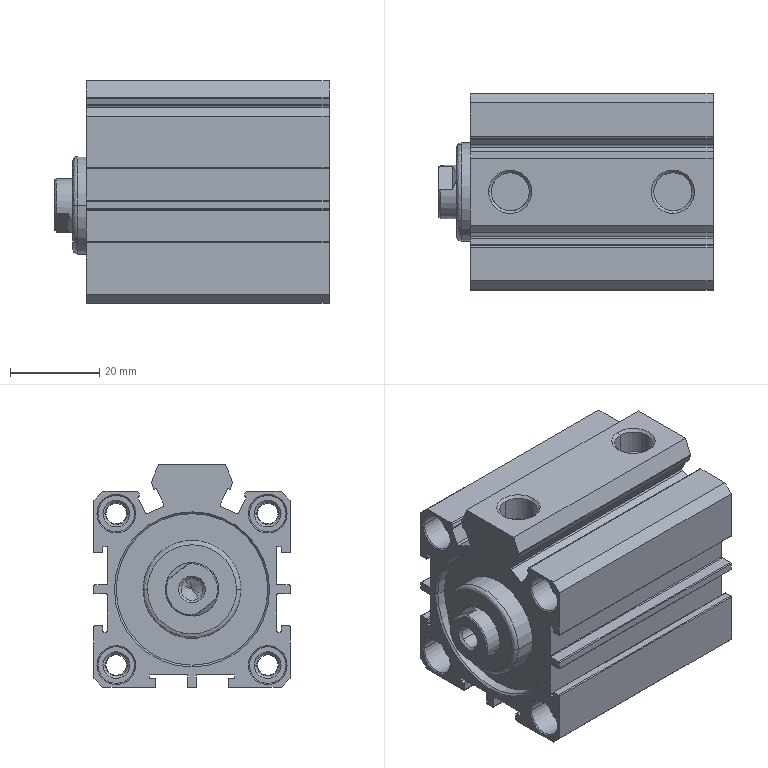Part | SolidWorks | 2 solids | 274 faces | box 61.5 x 44 x 50 mm | volume 72597 mm3 | cylinder 116 | plane 94 | cone 62 | spline 2 | commonest cylinder face diameters 0.4 x46 4.917 x18 8.2 x16 0.8 x10 4.6 x8 8.566 x4